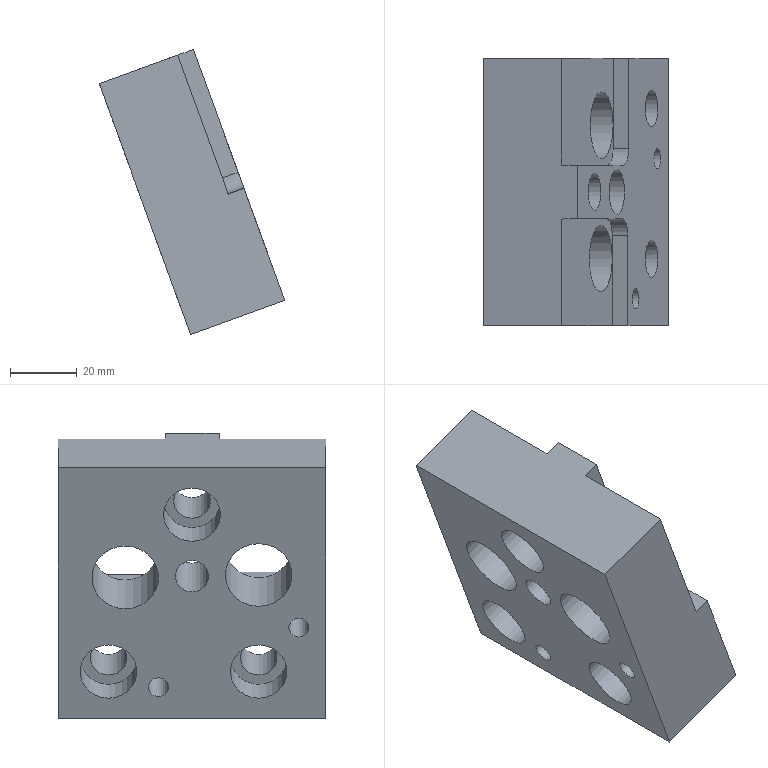Part | NX | features solid 2 | 1 solid | 30 faces | box 55.556 x 80.011 x 85.442 mm | volume 144406 mm3 | plane 16 | cylinder 14 | commonest cylinder face diameters 10 x3 11 x3 17 x3 6 x2 20 x2 13.5 x1
STEP:
#1=CARTESIAN_POINT('',(706.024,-306.997,52.44));
#2=VERTEX_POINT('',#1);
#3=CARTESIAN_POINT('',(703.117,-306.997,60.427));
#4=DIRECTION('',(0.9397,-0.000001517,0.342));
#5=DIRECTION('',(0.342,0.,-0.9397));
#6=AXIS2_PLACEMENT_3D('',#3,#4,#5);
#7=CIRCLE('',#6,8.5);
#8=EDGE_CURVE('',#2,#2,#7,.T.);
#9=ORIENTED_EDGE('',*,*,#8,.T.);
#10=EDGE_LOOP('',(#9));
#11=FACE_BOUND('',#10,.T.);
#12=CARTESIAN_POINT('',(717.31,-281.99,21.433));
#13=VERTEX_POINT('',#12);
#14=CARTESIAN_POINT('',(720.217,-281.99,13.446));
#15=DIRECTION('',(-0.9397,0.000001517,-0.342));
#16=DIRECTION('',(-0.342,0.00000071,0.9397));
#17=AXIS2_PLACEMENT_3D('',#14,#15,#16);
#18=CIRCLE('',#17,8.5);
#19=EDGE_CURVE('',#13,#13,#18,.T.);
#20=ORIENTED_EDGE('',*,*,#19,.F.);
#21=EDGE_LOOP('',(#20));
#22=FACE_BOUND('',#21,.T.);
#23=CARTESIAN_POINT('',(717.312,-326.99,21.427));
#24=VERTEX_POINT('',#23);
#25=CARTESIAN_POINT('',(720.219,-326.99,13.44));
#26=DIRECTION('',(-0.9397,0.000001517,-0.342));
#27=DIRECTION('',(-0.342,0.00000071,0.9397));
#28=AXIS2_PLACEMENT_3D('',#25,#26,#27);
#29=CIRCLE('',#28,8.5);
#30=EDGE_CURVE('',#24,#24,#29,.T.);
#31=ORIENTED_EDGE('',*,*,#30,.F.);
#32=EDGE_LOOP('',(#31));
#33=FACE_BOUND('',#32,.T.);
#34=CARTESIAN_POINT('',(711.536,-306.988,37.297));
#35=VERTEX_POINT('',#34);
#36=CARTESIAN_POINT('',(709.825,-306.988,41.995));
#37=DIRECTION('',(0.9397,-0.000001517,0.342));
#38=DIRECTION('',(0.342,-0.00000071,-0.9397));
#39=AXIS2_PLACEMENT_3D('',#36,#37,#38);
#40=CIRCLE('',#39,5.);
#41=EDGE_CURVE('',#35,#35,#40,.F.);
#42=ORIENTED_EDGE('',*,*,#41,.F.);
#43=EDGE_LOOP('',(#42));
#44=FACE_BOUND('',#43,.T.);
#45=CARTESIAN_POINT('',(725.35,-346.988,-0.6581));
#46=VERTEX_POINT('',#45);
#47=CARTESIAN_POINT('',(697.988,-346.999,74.517));
#48=VERTEX_POINT('',#47);
#49=CARTESIAN_POINT('',(727.06,-346.987,-5.357));
#50=DIRECTION('',(-0.342,-0.0001374,0.9397));
#51=VECTOR('',#50,1000.);
#52=LINE('',#49,#51);
#53=EDGE_CURVE('',#46,#48,#52,.T.);
#54=ORIENTED_EDGE('',*,*,#53,.T.);
#55=CARTESIAN_POINT('',(697.985,-266.999,74.528));
#56=VERTEX_POINT('',#55);
#57=CARTESIAN_POINT('',(697.983,-236.999,74.532));
#58=DIRECTION('',(-0.00004556,1.,0.0001296));
#59=VECTOR('',#58,1000.);
#60=LINE('',#57,#59);
#61=EDGE_CURVE('',#48,#56,#60,.T.);
#62=ORIENTED_EDGE('',*,*,#61,.T.);
#63=CARTESIAN_POINT('',(725.346,-266.988,-0.6477));
#64=VERTEX_POINT('',#63);
#65=CARTESIAN_POINT('',(727.056,-266.987,-5.346));
#66=DIRECTION('',(0.342,0.0001374,-0.9397));
#67=VECTOR('',#66,1000.);
#68=LINE('',#65,#67);
#69=EDGE_CURVE('',#56,#64,#68,.T.);
#70=ORIENTED_EDGE('',*,*,#69,.T.);
#71=CARTESIAN_POINT('',(725.345,-236.988,-0.6438));
#72=DIRECTION('',(0.00004556,-1.,-0.0001296));
#73=VECTOR('',#72,1000.);
#74=LINE('',#71,#73);
#75=EDGE_CURVE('',#64,#46,#74,.T.);
#76=ORIENTED_EDGE('',*,*,#75,.T.);
#77=EDGE_LOOP('',(#54,#62,#70,#76));
#78=FACE_BOUND('',#77,.T.);
#79=CARTESIAN_POINT('',(713.377,-286.994,32.239));
#80=VERTEX_POINT('',#79);
#81=CARTESIAN_POINT('',(709.956,-286.994,41.636));
#82=DIRECTION('',(0.9397,-0.000001517,0.342));
#83=DIRECTION('',(0.342,-0.00000071,-0.9397));
#84=AXIS2_PLACEMENT_3D('',#81,#82,#83);
#85=CIRCLE('',#84,10.);
#86=EDGE_CURVE('',#80,#80,#85,.F.);
#87=ORIENTED_EDGE('',*,*,#86,.F.);
#88=EDGE_LOOP('',(#87));
#89=FACE_BOUND('',#88,.T.);
#90=CARTESIAN_POINT('',(713.111,-326.986,32.967));
#91=VERTEX_POINT('',#90);
#92=CARTESIAN_POINT('',(709.691,-326.986,42.364));
#93=DIRECTION('',(0.9397,-0.000001517,0.342));
#94=DIRECTION('',(0.342,-0.00000071,-0.9397));
#95=AXIS2_PLACEMENT_3D('',#92,#93,#94);
#96=CIRCLE('',#95,10.);
#97=EDGE_CURVE('',#91,#91,#96,.F.);
#98=ORIENTED_EDGE('',*,*,#97,.F.);
#99=EDGE_LOOP('',(#98));
#100=FACE_BOUND('',#99,.T.);
#101=CARTESIAN_POINT('',(722.954,-296.989,5.926));
#102=VERTEX_POINT('',#101);
#103=CARTESIAN_POINT('',(721.927,-296.989,8.745));
#104=DIRECTION('',(0.9397,-0.000001517,0.342));
#105=DIRECTION('',(0.342,0.,-0.9397));
#106=AXIS2_PLACEMENT_3D('',#103,#104,#105);
#107=CIRCLE('',#106,3.);
#108=EDGE_CURVE('',#102,#102,#107,.F.);
#109=ORIENTED_EDGE('',*,*,#108,.F.);
#110=EDGE_LOOP('',(#109));
#111=FACE_BOUND('',#110,.T.);
#112=CARTESIAN_POINT('',(716.457,-338.992,23.775));
#113=VERTEX_POINT('',#112);
#114=CARTESIAN_POINT('',(715.431,-338.992,26.594));
#115=DIRECTION('',(0.9397,-0.000001517,0.342));
#116=DIRECTION('',(0.342,0.,-0.9397));
#117=AXIS2_PLACEMENT_3D('',#114,#115,#116);
#118=CIRCLE('',#117,3.);
#119=EDGE_CURVE('',#113,#113,#118,.F.);
#120=ORIENTED_EDGE('',*,*,#119,.F.);
#121=EDGE_LOOP('',(#120));
#122=FACE_BOUND('',#121,.T.);
#123=CARTESIAN_POINT('',(727.055,-236.987,-5.342));
#124=DIRECTION('',(-0.9397,0.000001517,-0.342));
#125=DIRECTION('',(0.342,0.0001374,-0.9397));
#126=AXIS2_PLACEMENT_3D('',#123,#124,#125);
#127=PLANE('',#126);
#128=ADVANCED_FACE('',(#11,#22,#33,#44,#78,#89,#100,#111,#122),#127,.T.);
#129=CARTESIAN_POINT('',(736.63,-346.993,41.445));
#130=VERTEX_POINT('',#129);
#131=CARTESIAN_POINT('',(721.481,-346.999,83.068));
#132=VERTEX_POINT('',#131);
#133=CARTESIAN_POINT('',(750.552,-346.987,3.194));
#134=DIRECTION('',(-0.342,-0.0001374,0.9397));
#135=VECTOR('',#134,1000.);
#136=LINE('',#133,#135);
#137=EDGE_CURVE('',#130,#132,#136,.T.);
#138=ORIENTED_EDGE('',*,*,#137,.T.);
#139=CARTESIAN_POINT('',(730.878,-346.999,86.488));
#140=DIRECTION('',(-0.9397,0.000001517,-0.342));
#141=VECTOR('',#140,1000.);
#142=LINE('',#139,#141);
#143=EDGE_CURVE('',#132,#48,#142,.T.);
#144=ORIENTED_EDGE('',*,*,#143,.T.);
#145=ORIENTED_EDGE('',*,*,#53,.F.);
#146=CARTESIAN_POINT('',(753.541,-346.988,9.603));
#147=VERTEX_POINT('',#146);
#148=CARTESIAN_POINT('',(758.239,-346.988,11.313));
#149=DIRECTION('',(-0.9397,0.000001517,-0.342));
#150=VECTOR('',#149,1000.);
#151=LINE('',#148,#150);
#152=EDGE_CURVE('',#147,#46,#151,.T.);
#153=ORIENTED_EDGE('',*,*,#152,.F.);
#154=CARTESIAN_POINT('',(741.328,-346.993,43.155));
#155=VERTEX_POINT('',#154);
#156=CARTESIAN_POINT('',(755.251,-346.987,4.904));
#157=DIRECTION('',(0.342,0.0001374,-0.9397));
#158=VECTOR('',#157,1000.);
#159=LINE('',#156,#158);
#160=EDGE_CURVE('',#155,#147,#159,.T.);
#161=ORIENTED_EDGE('',*,*,#160,.F.);
#162=CARTESIAN_POINT('',(736.63,-346.993,41.445));
#163=DIRECTION('',(0.9397,-0.000001517,0.342));
#164=VECTOR('',#163,1000.);
#165=LINE('',#162,#164);
#166=EDGE_CURVE('',#155,#130,#165,.F.);
#167=ORIENTED_EDGE('',*,*,#166,.T.);
#168=EDGE_LOOP('',(#138,#144,#145,#153,#161,#167));
#169=FACE_BOUND('',#168,.T.);
#170=CARTESIAN_POINT('',(759.949,-346.987,6.614));
#171=DIRECTION('',(0.00004556,-1.,-0.0001296));
#172=DIRECTION('',(0.9397,-0.000001517,0.342));
#173=AXIS2_PLACEMENT_3D('',#170,#171,#172);
#174=PLANE('',#173);
#175=ADVANCED_FACE('',(#169),#174,.T.);
#176=CARTESIAN_POINT('',(721.479,-315.154,83.072));
#177=VERTEX_POINT('',#176);
#178=CARTESIAN_POINT('',(721.476,-236.999,83.082));
#179=DIRECTION('',(-0.00004556,1.,0.0001296));
#180=VECTOR('',#179,1000.);
#181=LINE('',#178,#180);
#182=EDGE_CURVE('',#132,#177,#181,.T.);
#183=ORIENTED_EDGE('',*,*,#182,.T.);
#184=CARTESIAN_POINT('',(726.178,-315.154,84.782));
#185=VERTEX_POINT('',#184);
#186=CARTESIAN_POINT('',(730.876,-315.154,86.492));
#187=DIRECTION('',(-0.9397,0.000001517,-0.342));
#188=VECTOR('',#187,1000.);
#189=LINE('',#186,#188);
#190=EDGE_CURVE('',#177,#185,#189,.F.);
#191=ORIENTED_EDGE('',*,*,#190,.T.);
#192=CARTESIAN_POINT('',(726.177,-298.999,84.784));
#193=VERTEX_POINT('',#192);
#194=CARTESIAN_POINT('',(726.174,-236.999,84.792));
#195=DIRECTION('',(0.00004556,-1.,-0.0001296));
#196=VECTOR('',#195,1000.);
#197=LINE('',#194,#196);
#198=EDGE_CURVE('',#193,#185,#197,.T.);
#199=ORIENTED_EDGE('',*,*,#198,.F.);
#200=CARTESIAN_POINT('',(721.479,-298.999,83.074));
#201=VERTEX_POINT('',#200);
#202=CARTESIAN_POINT('',(730.875,-298.999,86.494));
#203=DIRECTION('',(-0.9397,0.000001517,-0.342));
#204=VECTOR('',#203,1000.);
#205=LINE('',#202,#204);
#206=EDGE_CURVE('',#193,#201,#205,.T.);
#207=ORIENTED_EDGE('',*,*,#206,.T.);
#208=CARTESIAN_POINT('',(721.477,-266.999,83.078));
#209=VERTEX_POINT('',#208);
#210=CARTESIAN_POINT('',(721.476,-236.999,83.082));
#211=DIRECTION('',(-0.00004556,1.,0.0001296));
#212=VECTOR('',#211,1000.);
#213=LINE('',#210,#212);
#214=EDGE_CURVE('',#201,#209,#213,.T.);
#215=ORIENTED_EDGE('',*,*,#214,.T.);
#216=CARTESIAN_POINT('',(730.874,-266.999,86.498));
#217=DIRECTION('',(-0.9397,0.000001517,-0.342));
#218=VECTOR('',#217,1000.);
#219=LINE('',#216,#218);
#220=EDGE_CURVE('',#209,#56,#219,.T.);
#221=ORIENTED_EDGE('',*,*,#220,.T.);
#222=ORIENTED_EDGE('',*,*,#61,.F.);
#223=ORIENTED_EDGE('',*,*,#143,.F.);
#224=EDGE_LOOP('',(#183,#191,#199,#207,#215,#221,#222,#223));
#225=FACE_BOUND('',#224,.T.);
#226=CARTESIAN_POINT('',(730.873,-236.999,86.502));
#227=DIRECTION('',(-0.342,-0.0001374,0.9397));
#228=DIRECTION('',(-0.9397,0.000001517,-0.342));
#229=AXIS2_PLACEMENT_3D('',#226,#227,#228);
#230=PLANE('',#229);
#231=ADVANCED_FACE('',(#225),#230,.T.);
#232=CARTESIAN_POINT('',(736.868,-266.993,40.792));
#233=VERTEX_POINT('',#232);
#234=CARTESIAN_POINT('',(750.549,-266.987,3.204));
#235=DIRECTION('',(0.342,0.0001374,-0.9397));
#236=VECTOR('',#235,1000.);
#237=LINE('',#234,#236);
#238=EDGE_CURVE('',#209,#233,#237,.T.);
#239=ORIENTED_EDGE('',*,*,#238,.T.);
#240=CARTESIAN_POINT('',(741.566,-266.993,42.502));
#241=VERTEX_POINT('',#240);
#242=CARTESIAN_POINT('',(746.265,-266.993,44.212));
#243=DIRECTION('',(0.9397,-0.000001517,0.342));
#244=VECTOR('',#243,1000.);
#245=LINE('',#242,#244);
#246=EDGE_CURVE('',#233,#241,#245,.T.);
#247=ORIENTED_EDGE('',*,*,#246,.T.);
#248=CARTESIAN_POINT('',(753.537,-266.988,9.613));
#249=VERTEX_POINT('',#248);
#250=CARTESIAN_POINT('',(755.247,-266.987,4.914));
#251=DIRECTION('',(-0.342,-0.0001374,0.9397));
#252=VECTOR('',#251,1000.);
#253=LINE('',#250,#252);
#254=EDGE_CURVE('',#249,#241,#253,.T.);
#255=ORIENTED_EDGE('',*,*,#254,.F.);
#256=CARTESIAN_POINT('',(758.236,-266.988,11.323));
#257=DIRECTION('',(-0.9397,0.000001517,-0.342));
#258=VECTOR('',#257,1000.);
#259=LINE('',#256,#258);
#260=EDGE_CURVE('',#249,#64,#259,.T.);
#261=ORIENTED_EDGE('',*,*,#260,.T.);
#262=ORIENTED_EDGE('',*,*,#69,.F.);
#263=ORIENTED_EDGE('',*,*,#220,.F.);
#264=EDGE_LOOP('',(#239,#247,#255,#261,#262,#263));
#265=FACE_BOUND('',#264,.T.);
#266=CARTESIAN_POINT('',(759.946,-266.987,6.625));
#267=DIRECTION('',(-0.00004556,1.,0.0001296));
#268=DIRECTION('',(-0.9397,0.000001517,-0.342));
#269=AXIS2_PLACEMENT_3D('',#266,#267,#268);
#270=PLANE('',#269);
#271=ADVANCED_FACE('',(#265),#270,.T.);
#272=CARTESIAN_POINT('',(729.427,-306.997,75.856));
#273=VERTEX_POINT('',#272);
#274=CARTESIAN_POINT('',(731.308,-306.997,70.688));
#275=DIRECTION('',(-0.9397,0.000001517,-0.342));
#276=DIRECTION('',(-0.342,0.,0.9397));
#277=AXIS2_PLACEMENT_3D('',#274,#275,#276);
#278=CIRCLE('',#277,5.5);
#279=EDGE_CURVE('',#273,#273,#278,.T.);
#280=ORIENTED_EDGE('',*,*,#279,.T.);
#281=EDGE_LOOP('',(#280));
#282=FACE_BOUND('',#281,.T.);
#283=CARTESIAN_POINT('',(742.596,-338.992,39.674));
#284=VERTEX_POINT('',#283);
#285=CARTESIAN_POINT('',(743.622,-338.992,36.855));
#286=DIRECTION('',(-0.9397,0.000001517,-0.342));
#287=DIRECTION('',(-0.342,0.00000071,0.9397));
#288=AXIS2_PLACEMENT_3D('',#285,#286,#287);
#289=CIRCLE('',#288,3.);
#290=EDGE_CURVE('',#284,#284,#289,.T.);
#291=ORIENTED_EDGE('',*,*,#290,.T.);
#292=EDGE_LOOP('',(#291));
#293=FACE_BOUND('',#292,.T.);
#294=CARTESIAN_POINT('',(749.092,-296.989,21.825));
#295=VERTEX_POINT('',#294);
#296=CARTESIAN_POINT('',(750.118,-296.989,19.006));
#297=DIRECTION('',(-0.9397,0.000001517,-0.342));
#298=DIRECTION('',(-0.342,0.00000071,0.9397));
#299=AXIS2_PLACEMENT_3D('',#296,#297,#298);
#300=CIRCLE('',#299,3.);
#301=EDGE_CURVE('',#295,#295,#300,.T.);
#302=ORIENTED_EDGE('',*,*,#301,.T.);
#303=EDGE_LOOP('',(#302));
#304=FACE_BOUND('',#303,.T.);
#305=CARTESIAN_POINT('',(746.526,-281.99,28.875));
#306=VERTEX_POINT('',#305);
#307=CARTESIAN_POINT('',(748.407,-281.99,23.706));
#308=DIRECTION('',(-0.9397,0.000001517,-0.342));
#309=DIRECTION('',(-0.342,0.00000071,0.9397));
#310=AXIS2_PLACEMENT_3D('',#307,#308,#309);
#311=CIRCLE('',#310,5.5);
#312=EDGE_CURVE('',#306,#306,#311,.T.);
#313=ORIENTED_EDGE('',*,*,#312,.T.);
#314=EDGE_LOOP('',(#313));
#315=FACE_BOUND('',#314,.T.);
#316=CARTESIAN_POINT('',(746.528,-326.99,28.869));
#317=VERTEX_POINT('',#316);
#318=CARTESIAN_POINT('',(748.41,-326.99,23.701));
#319=DIRECTION('',(-0.9397,0.000001517,-0.342));
#320=DIRECTION('',(-0.342,0.00000071,0.9397));
#321=AXIS2_PLACEMENT_3D('',#318,#319,#320);
#322=CIRCLE('',#321,5.5);
#323=EDGE_CURVE('',#317,#317,#322,.T.);
#324=ORIENTED_EDGE('',*,*,#323,.T.);
#325=EDGE_LOOP('',(#324));
#326=FACE_BOUND('',#325,.T.);
#327=ORIENTED_EDGE('',*,*,#160,.T.);
#328=CARTESIAN_POINT('',(753.536,-236.988,9.617));
#329=DIRECTION('',(-0.00004556,1.,0.0001296));
#330=VECTOR('',#329,1000.);
#331=LINE('',#328,#330);
#332=EDGE_CURVE('',#147,#249,#331,.T.);
#333=ORIENTED_EDGE('',*,*,#332,.T.);
#334=ORIENTED_EDGE('',*,*,#254,.T.);
#335=CARTESIAN_POINT('',(741.568,-293.993,42.499));
#336=VERTEX_POINT('',#335);
#337=CARTESIAN_POINT('',(741.565,-236.993,42.506));
#338=DIRECTION('',(0.00004556,-1.,-0.0001296));
#339=VECTOR('',#338,1000.);
#340=LINE('',#337,#339);
#341=EDGE_CURVE('',#241,#336,#340,.T.);
#342=ORIENTED_EDGE('',*,*,#341,.T.);
#343=CARTESIAN_POINT('',(739.858,-298.993,47.196));
#344=VERTEX_POINT('',#343);
#345=CARTESIAN_POINT('',(739.858,-293.993,47.197));
#346=DIRECTION('',(-0.9397,0.000001517,-0.342));
#347=DIRECTION('',(-0.342,0.00000071,0.9397));
#348=AXIS2_PLACEMENT_3D('',#345,#346,#347);
#349=CIRCLE('',#348,5.);
#350=EDGE_CURVE('',#344,#336,#349,.F.);
#351=ORIENTED_EDGE('',*,*,#350,.F.);
#352=CARTESIAN_POINT('',(755.249,-298.987,4.91));
#353=DIRECTION('',(-0.342,-0.0001374,0.9397));
#354=VECTOR('',#353,1000.);
#355=LINE('',#352,#354);
#356=EDGE_CURVE('',#344,#193,#355,.T.);
#357=ORIENTED_EDGE('',*,*,#356,.T.);
#358=ORIENTED_EDGE('',*,*,#198,.T.);
#359=CARTESIAN_POINT('',(739.576,-315.004,47.969));
#360=VERTEX_POINT('',#359);
#361=CARTESIAN_POINT('',(755.348,-314.827,4.638));
#362=DIRECTION('',(-0.342,-0.003837,0.9397));
#363=VECTOR('',#362,1000.);
#364=LINE('',#361,#363);
#365=EDGE_CURVE('',#185,#360,#364,.F.);
#366=ORIENTED_EDGE('',*,*,#365,.T.);
#367=CARTESIAN_POINT('',(741.293,-319.985,43.253));
#368=VERTEX_POINT('',#367);
#369=CARTESIAN_POINT('',(739.583,-320.004,47.951));
#370=DIRECTION('',(-0.9397,0.000001517,-0.342));
#371=DIRECTION('',(-0.342,0.00000071,0.9397));
#372=AXIS2_PLACEMENT_3D('',#369,#370,#371);
#373=CIRCLE('',#372,5.);
#374=EDGE_CURVE('',#368,#360,#373,.F.);
#375=ORIENTED_EDGE('',*,*,#374,.F.);
#376=CARTESIAN_POINT('',(741.275,-306.392,43.302));
#377=DIRECTION('',(-0.001311,1.,0.003606));
#378=VECTOR('',#377,1000.);
#379=LINE('',#376,#378);
#380=EDGE_CURVE('',#368,#155,#379,.F.);
#381=ORIENTED_EDGE('',*,*,#380,.T.);
#382=EDGE_LOOP('',(#327,#333,#334,#342,#351,#357,#358,#366,#375,#381));
#383=FACE_BOUND('',#382,.T.);
#384=CARTESIAN_POINT('',(735.708,-306.989,58.599));
#385=VERTEX_POINT('',#384);
#386=CARTESIAN_POINT('',(738.016,-306.989,52.256));
#387=DIRECTION('',(-0.9397,0.000001517,-0.342));
#388=DIRECTION('',(-0.342,0.00000071,0.9397));
#389=AXIS2_PLACEMENT_3D('',#386,#387,#388);
#390=CIRCLE('',#389,6.75);
#391=EDGE_CURVE('',#385,#385,#390,.T.);
#392=ORIENTED_EDGE('',*,*,#391,.T.);
#393=EDGE_LOOP('',(#392));
#394=FACE_BOUND('',#393,.T.);
#395=CARTESIAN_POINT('',(755.246,-236.987,4.918));
#396=DIRECTION('',(0.9397,-0.000001517,0.342));
#397=DIRECTION('',(-0.342,-0.0001374,0.9397));
#398=AXIS2_PLACEMENT_3D('',#395,#396,#397);
#399=PLANE('',#398);
#400=ADVANCED_FACE('',(#282,#293,#304,#315,#326,#383,#394),#399,.T.);
#401=ORIENTED_EDGE('',*,*,#332,.F.);
#402=ORIENTED_EDGE('',*,*,#152,.T.);
#403=ORIENTED_EDGE('',*,*,#75,.F.);
#404=ORIENTED_EDGE('',*,*,#260,.F.);
#405=EDGE_LOOP('',(#401,#402,#403,#404));
#406=FACE_BOUND('',#405,.T.);
#407=CARTESIAN_POINT('',(758.234,-236.988,11.327));
#408=DIRECTION('',(0.342,0.0001374,-0.9397));
#409=DIRECTION('',(0.9397,-0.000001517,0.342));
#410=AXIS2_PLACEMENT_3D('',#407,#408,#409);
#411=PLANE('',#410);
#412=ADVANCED_FACE('',(#406),#411,.T.);
#413=CARTESIAN_POINT('',(736.869,-286.993,40.789));
#414=VERTEX_POINT('',#413);
#415=CARTESIAN_POINT('',(736.869,-293.993,40.789));
#416=VERTEX_POINT('',#415);
#417=CARTESIAN_POINT('',(736.869,-281.993,40.79));
#418=DIRECTION('',(0.00004556,-1.,-0.0001296));
#419=VECTOR('',#418,1000.);
#420=LINE('',#417,#419);
#421=EDGE_CURVE('',#414,#416,#420,.T.);
#422=ORIENTED_EDGE('',*,*,#421,.F.);
#423=CARTESIAN_POINT('',(733.449,-286.994,50.186));
#424=DIRECTION('',(-0.9397,0.000001517,-0.342));
#425=DIRECTION('',(-0.342,-0.0001374,0.9397));
#426=AXIS2_PLACEMENT_3D('',#423,#424,#425);
#427=CIRCLE('',#426,10.);
#428=EDGE_CURVE('',#414,#414,#427,.T.);
#429=ORIENTED_EDGE('',*,*,#428,.T.);
#430=CARTESIAN_POINT('',(736.869,-281.993,40.79));
#431=DIRECTION('',(0.00004556,-1.,-0.0001296));
#432=VECTOR('',#431,1000.);
#433=LINE('',#430,#432);
#434=EDGE_CURVE('',#233,#414,#433,.T.);
#435=ORIENTED_EDGE('',*,*,#434,.F.);
#436=ORIENTED_EDGE('',*,*,#238,.F.);
#437=ORIENTED_EDGE('',*,*,#214,.F.);
#438=CARTESIAN_POINT('',(735.159,-298.993,45.486));
#439=VERTEX_POINT('',#438);
#440=CARTESIAN_POINT('',(735.159,-298.993,45.486));
#441=DIRECTION('',(-0.342,-0.0001374,0.9397));
#442=VECTOR('',#441,1000.);
#443=LINE('',#440,#442);
#444=EDGE_CURVE('',#439,#201,#443,.T.);
#445=ORIENTED_EDGE('',*,*,#444,.F.);
#446=CARTESIAN_POINT('',(735.159,-293.993,45.487));
#447=DIRECTION('',(0.9397,-0.000001517,0.342));
#448=DIRECTION('',(0.342,-0.00000071,-0.9397));
#449=AXIS2_PLACEMENT_3D('',#446,#447,#448);
#450=CIRCLE('',#449,5.);
#451=EDGE_CURVE('',#416,#439,#450,.F.);
#452=ORIENTED_EDGE('',*,*,#451,.F.);
#453=EDGE_LOOP('',(#422,#429,#435,#436,#437,#445,#452));
#454=FACE_BOUND('',#453,.T.);
#455=CARTESIAN_POINT('',(735.159,-281.993,45.489));
#456=DIRECTION('',(-0.9397,0.000001517,-0.342));
#457=DIRECTION('',(0.342,0.0001374,-0.9397));
#458=AXIS2_PLACEMENT_3D('',#455,#456,#457);
#459=PLANE('',#458);
#460=ADVANCED_FACE('',(#454),#459,.F.);
#461=ORIENTED_EDGE('',*,*,#444,.T.);
#462=ORIENTED_EDGE('',*,*,#206,.F.);
#463=ORIENTED_EDGE('',*,*,#356,.F.);
#464=CARTESIAN_POINT('',(739.858,-298.993,47.196));
#465=DIRECTION('',(-0.9397,0.000001517,-0.342));
#466=VECTOR('',#465,1000.);
#467=LINE('',#464,#466);
#468=EDGE_CURVE('',#439,#344,#467,.F.);
#469=ORIENTED_EDGE('',*,*,#468,.F.);
#470=EDGE_LOOP('',(#461,#462,#463,#469));
#471=FACE_BOUND('',#470,.T.);
#472=CARTESIAN_POINT('',(739.858,-298.993,47.196));
#473=DIRECTION('',(0.00004556,-1.,-0.0001296));
#474=DIRECTION('',(0.9397,-0.000001517,0.342));
#475=AXIS2_PLACEMENT_3D('',#472,#473,#474);
#476=PLANE('',#475);
#477=ADVANCED_FACE('',(#471),#476,.F.);
#478=ORIENTED_EDGE('',*,*,#341,.F.);
#479=ORIENTED_EDGE('',*,*,#246,.F.);
#480=ORIENTED_EDGE('',*,*,#434,.T.);
#481=ORIENTED_EDGE('',*,*,#421,.T.);
#482=CARTESIAN_POINT('',(736.869,-293.993,40.789));
#483=DIRECTION('',(-0.9397,0.000001517,-0.342));
#484=VECTOR('',#483,1000.);
#485=LINE('',#482,#484);
#486=EDGE_CURVE('',#336,#416,#485,.T.);
#487=ORIENTED_EDGE('',*,*,#486,.F.);
#488=EDGE_LOOP('',(#478,#479,#480,#481,#487));
#489=FACE_BOUND('',#488,.T.);
#490=CARTESIAN_POINT('',(741.567,-281.993,42.5));
#491=DIRECTION('',(0.342,0.0001374,-0.9397));
#492=DIRECTION('',(0.9397,-0.000001517,0.342));
#493=AXIS2_PLACEMENT_3D('',#490,#491,#492);
#494=PLANE('',#493);
#495=ADVANCED_FACE('',(#489),#494,.F.);
#496=CARTESIAN_POINT('',(734.878,-315.004,46.259));
#497=VERTEX_POINT('',#496);
#498=CARTESIAN_POINT('',(736.588,-314.985,41.561));
#499=DIRECTION('',(-0.342,-0.003837,0.9397));
#500=VECTOR('',#499,1000.);
#501=LINE('',#498,#500);
#502=EDGE_CURVE('',#177,#497,#501,.F.);
#503=ORIENTED_EDGE('',*,*,#502,.F.);
#504=ORIENTED_EDGE('',*,*,#182,.F.);
#505=ORIENTED_EDGE('',*,*,#137,.F.);
#506=CARTESIAN_POINT('',(736.604,-326.948,41.518));
#507=VERTEX_POINT('',#506);
#508=CARTESIAN_POINT('',(736.597,-321.966,41.536));
#509=DIRECTION('',(-0.001311,1.,0.003606));
#510=VECTOR('',#509,1000.);
#511=LINE('',#508,#510);
#512=EDGE_CURVE('',#507,#130,#511,.F.);
#513=ORIENTED_EDGE('',*,*,#512,.F.);
#514=CARTESIAN_POINT('',(733.184,-326.986,50.914));
#515=DIRECTION('',(-0.9397,0.000001517,-0.342));
#516=DIRECTION('',(-0.342,-0.003837,0.9397));
#517=AXIS2_PLACEMENT_3D('',#514,#515,#516);
#518=CIRCLE('',#517,10.);
#519=EDGE_CURVE('',#507,#507,#518,.T.);
#520=ORIENTED_EDGE('',*,*,#519,.T.);
#521=CARTESIAN_POINT('',(736.595,-319.985,41.543));
#522=VERTEX_POINT('',#521);
#523=CARTESIAN_POINT('',(736.597,-321.966,41.536));
#524=DIRECTION('',(-0.001311,1.,0.003606));
#525=VECTOR('',#524,1000.);
#526=LINE('',#523,#525);
#527=EDGE_CURVE('',#522,#507,#526,.F.);
#528=ORIENTED_EDGE('',*,*,#527,.F.);
#529=CARTESIAN_POINT('',(734.885,-320.004,46.241));
#530=DIRECTION('',(0.9397,-0.000001517,0.342));
#531=DIRECTION('',(0.342,-0.00000071,-0.9397));
#532=AXIS2_PLACEMENT_3D('',#529,#530,#531);
#533=CIRCLE('',#532,5.);
#534=EDGE_CURVE('',#497,#522,#533,.F.);
#535=ORIENTED_EDGE('',*,*,#534,.F.);
#536=EDGE_LOOP('',(#503,#504,#505,#513,#520,#528,#535));
#537=FACE_BOUND('',#536,.T.);
#538=CARTESIAN_POINT('',(734.893,-321.985,46.217));
#539=DIRECTION('',(-0.9397,0.000001517,-0.342));
#540=DIRECTION('',(0.342,0.0001374,-0.9397));
#541=AXIS2_PLACEMENT_3D('',#538,#539,#540);
#542=PLANE('',#541);
#543=ADVANCED_FACE('',(#537),#542,.F.);
#544=ORIENTED_EDGE('',*,*,#365,.F.);
#545=ORIENTED_EDGE('',*,*,#190,.F.);
#546=ORIENTED_EDGE('',*,*,#502,.T.);
#547=CARTESIAN_POINT('',(734.878,-315.004,46.259));
#548=DIRECTION('',(0.9397,-0.000001517,0.342));
#549=VECTOR('',#548,1000.);
#550=LINE('',#547,#549);
#551=EDGE_CURVE('',#360,#497,#550,.F.);
#552=ORIENTED_EDGE('',*,*,#551,.F.);
#553=EDGE_LOOP('',(#544,#545,#546,#552));
#554=FACE_BOUND('',#553,.T.);
#555=CARTESIAN_POINT('',(736.588,-314.985,41.561));
#556=DIRECTION('',(0.001311,-1.,-0.003606));
#557=DIRECTION('',(-0.000000496,0.003606,-1.));
#558=AXIS2_PLACEMENT_3D('',#555,#556,#557);
#559=PLANE('',#558);
#560=ADVANCED_FACE('',(#554),#559,.T.);
#561=ORIENTED_EDGE('',*,*,#527,.T.);
#562=ORIENTED_EDGE('',*,*,#512,.T.);
#563=ORIENTED_EDGE('',*,*,#166,.F.);
#564=ORIENTED_EDGE('',*,*,#380,.F.);
#565=CARTESIAN_POINT('',(736.595,-319.985,41.543));
#566=DIRECTION('',(0.9397,-0.000001517,0.342));
#567=VECTOR('',#566,1000.);
#568=LINE('',#565,#567);
#569=EDGE_CURVE('',#522,#368,#568,.T.);
#570=ORIENTED_EDGE('',*,*,#569,.F.);
#571=EDGE_LOOP('',(#561,#562,#563,#564,#570));
#572=FACE_BOUND('',#571,.T.);
#573=CARTESIAN_POINT('',(736.577,-306.392,41.592));
#574=DIRECTION('',(0.342,0.003837,-0.9397));
#575=DIRECTION('',(0.001311,-1.,-0.003606));
#576=AXIS2_PLACEMENT_3D('',#573,#574,#575);
#577=PLANE('',#576);
#578=ADVANCED_FACE('',(#572),#577,.F.);
#579=ORIENTED_EDGE('',*,*,#391,.F.);
#580=EDGE_LOOP('',(#579));
#581=FACE_BOUND('',#580,.T.);
#582=CARTESIAN_POINT('',(735.626,-306.989,44.203));
#583=VERTEX_POINT('',#582);
#584=CARTESIAN_POINT('',(733.318,-306.989,50.546));
#585=DIRECTION('',(0.9397,-0.000001517,0.342));
#586=DIRECTION('',(0.342,-0.00000071,-0.9397));
#587=AXIS2_PLACEMENT_3D('',#584,#585,#586);
#588=CIRCLE('',#587,6.75);
#589=EDGE_CURVE('',#583,#583,#588,.T.);
#590=ORIENTED_EDGE('',*,*,#589,.F.);
#591=EDGE_LOOP('',(#590));
#592=FACE_BOUND('',#591,.T.);
#593=CARTESIAN_POINT('',(742.715,-306.989,53.966));
#594=DIRECTION('',(-0.9397,0.000001517,-0.342));
#595=DIRECTION('',(0.342,-0.00000071,-0.9397));
#596=AXIS2_PLACEMENT_3D('',#593,#594,#595);
#597=CYLINDRICAL_SURFACE('',#596,6.75);
#598=ADVANCED_FACE('',(#581,#592),#597,.F.);
#599=ORIENTED_EDGE('',*,*,#589,.T.);
#600=EDGE_LOOP('',(#599));
#601=FACE_BOUND('',#600,.T.);
#602=CARTESIAN_POINT('',(731.608,-306.989,55.244));
#603=VERTEX_POINT('',#602);
#604=CARTESIAN_POINT('',(733.318,-306.989,50.546));
#605=DIRECTION('',(-0.9397,0.000001517,-0.342));
#606=DIRECTION('',(-0.342,0.00000071,0.9397));
#607=AXIS2_PLACEMENT_3D('',#604,#605,#606);
#608=CIRCLE('',#607,5.);
#609=EDGE_CURVE('',#603,#603,#608,.T.);
#610=ORIENTED_EDGE('',*,*,#609,.T.);
#611=EDGE_LOOP('',(#610));
#612=FACE_BOUND('',#611,.T.);
#613=CARTESIAN_POINT('',(733.318,-306.989,50.546));
#614=DIRECTION('',(-0.9397,0.000001517,-0.342));
#615=DIRECTION('',(0.342,-0.00000071,-0.9397));
#616=AXIS2_PLACEMENT_3D('',#613,#614,#615);
#617=PLANE('',#616);
#618=ADVANCED_FACE('',(#601,#612),#617,.F.);
#619=ORIENTED_EDGE('',*,*,#86,.T.);
#620=EDGE_LOOP('',(#619));
#621=FACE_BOUND('',#620,.T.);
#622=ORIENTED_EDGE('',*,*,#428,.F.);
#623=EDGE_LOOP('',(#622));
#624=FACE_BOUND('',#623,.T.);
#625=CARTESIAN_POINT('',(738.147,-286.994,51.896));
#626=DIRECTION('',(-0.9397,0.000001517,-0.342));
#627=DIRECTION('',(0.342,0.0001374,-0.9397));
#628=AXIS2_PLACEMENT_3D('',#625,#626,#627);
#629=CYLINDRICAL_SURFACE('',#628,10.);
#630=ADVANCED_FACE('',(#621,#624),#629,.F.);
#631=ORIENTED_EDGE('',*,*,#41,.T.);
#632=EDGE_LOOP('',(#631));
#633=FACE_BOUND('',#632,.T.);
#634=ORIENTED_EDGE('',*,*,#609,.F.);
#635=EDGE_LOOP('',(#634));
#636=FACE_BOUND('',#635,.T.);
#637=CARTESIAN_POINT('',(738.016,-306.989,52.256));
#638=DIRECTION('',(-0.9397,0.000001517,-0.342));
#639=DIRECTION('',(0.342,-0.00000071,-0.9397));
#640=AXIS2_PLACEMENT_3D('',#637,#638,#639);
#641=CYLINDRICAL_SURFACE('',#640,5.);
#642=ADVANCED_FACE('',(#633,#636),#641,.F.);
#643=ORIENTED_EDGE('',*,*,#97,.T.);
#644=EDGE_LOOP('',(#643));
#645=FACE_BOUND('',#644,.T.);
#646=ORIENTED_EDGE('',*,*,#519,.F.);
#647=EDGE_LOOP('',(#646));
#648=FACE_BOUND('',#647,.T.);
#649=CARTESIAN_POINT('',(737.882,-326.986,52.625));
#650=DIRECTION('',(-0.9397,0.000001517,-0.342));
#651=DIRECTION('',(0.342,0.003837,-0.9397));
#652=AXIS2_PLACEMENT_3D('',#649,#650,#651);
#653=CYLINDRICAL_SURFACE('',#652,10.);
#654=ADVANCED_FACE('',(#645,#648),#653,.F.);
#655=ORIENTED_EDGE('',*,*,#323,.F.);
#656=EDGE_LOOP('',(#655));
#657=FACE_BOUND('',#656,.T.);
#658=CARTESIAN_POINT('',(729.614,-326.99,22.712));
#659=VERTEX_POINT('',#658);
#660=CARTESIAN_POINT('',(731.495,-326.99,17.544));
#661=DIRECTION('',(-0.9397,0.000001517,-0.342));
#662=DIRECTION('',(-0.342,0.00000071,0.9397));
#663=AXIS2_PLACEMENT_3D('',#660,#661,#662);
#664=CIRCLE('',#663,5.5);
#665=EDGE_CURVE('',#659,#659,#664,.T.);
#666=ORIENTED_EDGE('',*,*,#665,.T.);
#667=EDGE_LOOP('',(#666));
#668=FACE_BOUND('',#667,.T.);
#669=CARTESIAN_POINT('',(767.203,-326.99,30.541));
#670=DIRECTION('',(0.9397,-0.000001517,0.342));
#671=DIRECTION('',(-0.342,0.00000071,0.9397));
#672=AXIS2_PLACEMENT_3D('',#669,#670,#671);
#673=CYLINDRICAL_SURFACE('',#672,5.5);
#674=ADVANCED_FACE('',(#657,#668),#673,.F.);
#675=ORIENTED_EDGE('',*,*,#665,.F.);
#676=EDGE_LOOP('',(#675));
#677=FACE_BOUND('',#676,.T.);
#678=CARTESIAN_POINT('',(728.588,-326.99,25.532));
#679=VERTEX_POINT('',#678);
#680=CARTESIAN_POINT('',(731.495,-326.99,17.544));
#681=DIRECTION('',(-0.9397,0.000001517,-0.342));
#682=DIRECTION('',(-0.342,0.00000071,0.9397));
#683=AXIS2_PLACEMENT_3D('',#680,#681,#682);
#684=CIRCLE('',#683,8.5);
#685=EDGE_CURVE('',#679,#679,#684,.T.);
#686=ORIENTED_EDGE('',*,*,#685,.T.);
#687=EDGE_LOOP('',(#686));
#688=FACE_BOUND('',#687,.T.);
#689=CARTESIAN_POINT('',(731.495,-326.99,17.544));
#690=DIRECTION('',(0.9397,-0.000001517,0.342));
#691=DIRECTION('',(-0.342,0.00000071,0.9397));
#692=AXIS2_PLACEMENT_3D('',#689,#690,#691);
#693=PLANE('',#692);
#694=ADVANCED_FACE('',(#677,#688),#693,.F.);
#695=ORIENTED_EDGE('',*,*,#685,.F.);
#696=EDGE_LOOP('',(#695));
#697=FACE_BOUND('',#696,.T.);
#698=ORIENTED_EDGE('',*,*,#30,.T.);
#699=EDGE_LOOP('',(#698));
#700=FACE_BOUND('',#699,.T.);
#701=CARTESIAN_POINT('',(720.219,-326.99,13.44));
#702=DIRECTION('',(0.9397,-0.000001517,0.342));
#703=DIRECTION('',(-0.342,0.00000071,0.9397));
#704=AXIS2_PLACEMENT_3D('',#701,#702,#703);
#705=CYLINDRICAL_SURFACE('',#704,8.5);
#706=ADVANCED_FACE('',(#697,#700),#705,.F.);
#707=ORIENTED_EDGE('',*,*,#312,.F.);
#708=EDGE_LOOP('',(#707));
#709=FACE_BOUND('',#708,.T.);
#710=CARTESIAN_POINT('',(729.612,-281.99,22.718));
#711=VERTEX_POINT('',#710);
#712=CARTESIAN_POINT('',(731.493,-281.99,17.55));
#713=DIRECTION('',(-0.9397,0.000001517,-0.342));
#714=DIRECTION('',(-0.342,0.00000071,0.9397));
#715=AXIS2_PLACEMENT_3D('',#712,#713,#714);
#716=CIRCLE('',#715,5.5);
#717=EDGE_CURVE('',#711,#711,#716,.T.);
#718=ORIENTED_EDGE('',*,*,#717,.T.);
#719=EDGE_LOOP('',(#718));
#720=FACE_BOUND('',#719,.T.);
#721=CARTESIAN_POINT('',(767.201,-281.99,30.547));
#722=DIRECTION('',(0.9397,-0.000001517,0.342));
#723=DIRECTION('',(-0.342,0.00000071,0.9397));
#724=AXIS2_PLACEMENT_3D('',#721,#722,#723);
#725=CYLINDRICAL_SURFACE('',#724,5.5);
#726=ADVANCED_FACE('',(#709,#720),#725,.F.);
#727=ORIENTED_EDGE('',*,*,#717,.F.);
#728=EDGE_LOOP('',(#727));
#729=FACE_BOUND('',#728,.T.);
#730=CARTESIAN_POINT('',(728.586,-281.99,25.537));
#731=VERTEX_POINT('',#730);
#732=CARTESIAN_POINT('',(731.493,-281.99,17.55));
#733=DIRECTION('',(-0.9397,0.000001517,-0.342));
#734=DIRECTION('',(-0.342,0.00000071,0.9397));
#735=AXIS2_PLACEMENT_3D('',#732,#733,#734);
#736=CIRCLE('',#735,8.5);
#737=EDGE_CURVE('',#731,#731,#736,.T.);
#738=ORIENTED_EDGE('',*,*,#737,.T.);
#739=EDGE_LOOP('',(#738));
#740=FACE_BOUND('',#739,.T.);
#741=CARTESIAN_POINT('',(731.493,-281.99,17.55));
#742=DIRECTION('',(0.9397,-0.000001517,0.342));
#743=DIRECTION('',(-0.342,0.00000071,0.9397));
#744=AXIS2_PLACEMENT_3D('',#741,#742,#743);
#745=PLANE('',#744);
#746=ADVANCED_FACE('',(#729,#740),#745,.F.);
#747=ORIENTED_EDGE('',*,*,#737,.F.);
#748=EDGE_LOOP('',(#747));
#749=FACE_BOUND('',#748,.T.);
#750=ORIENTED_EDGE('',*,*,#19,.T.);
#751=EDGE_LOOP('',(#750));
#752=FACE_BOUND('',#751,.T.);
#753=CARTESIAN_POINT('',(720.217,-281.99,13.446));
#754=DIRECTION('',(0.9397,-0.000001517,0.342));
#755=DIRECTION('',(-0.342,0.00000071,0.9397));
#756=AXIS2_PLACEMENT_3D('',#753,#754,#755);
#757=CYLINDRICAL_SURFACE('',#756,8.5);
#758=ADVANCED_FACE('',(#749,#752),#757,.F.);
#759=ORIENTED_EDGE('',*,*,#301,.F.);
#760=EDGE_LOOP('',(#759));
#761=FACE_BOUND('',#760,.T.);
#762=ORIENTED_EDGE('',*,*,#108,.T.);
#763=EDGE_LOOP('',(#762));
#764=FACE_BOUND('',#763,.T.);
#765=CARTESIAN_POINT('',(768.912,-296.989,25.846));
#766=DIRECTION('',(0.9397,-0.000001517,0.342));
#767=DIRECTION('',(-0.342,0.00000071,0.9397));
#768=AXIS2_PLACEMENT_3D('',#765,#766,#767);
#769=CYLINDRICAL_SURFACE('',#768,3.);
#770=ADVANCED_FACE('',(#761,#764),#769,.F.);
#771=ORIENTED_EDGE('',*,*,#290,.F.);
#772=EDGE_LOOP('',(#771));
#773=FACE_BOUND('',#772,.T.);
#774=ORIENTED_EDGE('',*,*,#119,.T.);
#775=EDGE_LOOP('',(#774));
#776=FACE_BOUND('',#775,.T.);
#777=CARTESIAN_POINT('',(762.416,-338.992,43.695));
#778=DIRECTION('',(0.9397,-0.000001517,0.342));
#779=DIRECTION('',(-0.342,0.00000071,0.9397));
#780=AXIS2_PLACEMENT_3D('',#777,#778,#779);
#781=CYLINDRICAL_SURFACE('',#780,3.);
#782=ADVANCED_FACE('',(#773,#776),#781,.F.);
#783=ORIENTED_EDGE('',*,*,#350,.T.);
#784=ORIENTED_EDGE('',*,*,#486,.T.);
#785=ORIENTED_EDGE('',*,*,#451,.T.);
#786=ORIENTED_EDGE('',*,*,#468,.T.);
#787=EDGE_LOOP('',(#783,#784,#785,#786));
#788=FACE_BOUND('',#787,.T.);
#789=CARTESIAN_POINT('',(739.858,-293.993,47.197));
#790=DIRECTION('',(0.9397,-0.000001517,0.342));
#791=DIRECTION('',(-0.342,0.00000071,0.9397));
#792=AXIS2_PLACEMENT_3D('',#789,#790,#791);
#793=CYLINDRICAL_SURFACE('',#792,5.);
#794=ADVANCED_FACE('',(#788),#793,.F.);
#795=ORIENTED_EDGE('',*,*,#374,.T.);
#796=ORIENTED_EDGE('',*,*,#551,.T.);
#797=ORIENTED_EDGE('',*,*,#534,.T.);
#798=ORIENTED_EDGE('',*,*,#569,.T.);
#799=EDGE_LOOP('',(#795,#796,#797,#798));
#800=FACE_BOUND('',#799,.T.);
#801=CARTESIAN_POINT('',(734.885,-320.004,46.241));
#802=DIRECTION('',(-0.9397,0.000001517,-0.342));
#803=DIRECTION('',(0.342,-0.00000071,-0.9397));
#804=AXIS2_PLACEMENT_3D('',#801,#802,#803);
#805=CYLINDRICAL_SURFACE('',#804,5.);
#806=ADVANCED_FACE('',(#800),#805,.F.);
#807=ORIENTED_EDGE('',*,*,#279,.F.);
#808=EDGE_LOOP('',(#807));
#809=FACE_BOUND('',#808,.T.);
#810=CARTESIAN_POINT('',(712.512,-306.997,69.7));
#811=VERTEX_POINT('',#810);
#812=CARTESIAN_POINT('',(714.393,-306.997,64.531));
#813=DIRECTION('',(-0.9397,0.000001517,-0.342));
#814=DIRECTION('',(-0.342,0.,0.9397));
#815=AXIS2_PLACEMENT_3D('',#812,#813,#814);
#816=CIRCLE('',#815,5.5);
#817=EDGE_CURVE('',#811,#811,#816,.F.);
#818=ORIENTED_EDGE('',*,*,#817,.F.);
#819=EDGE_LOOP('',(#818));
#820=FACE_BOUND('',#819,.T.);
#821=CARTESIAN_POINT('',(748.222,-306.997,76.844));
#822=DIRECTION('',(-0.9397,0.000001517,-0.342));
#823=DIRECTION('',(0.342,0.,-0.9397));
#824=AXIS2_PLACEMENT_3D('',#821,#822,#823);
#825=CYLINDRICAL_SURFACE('',#824,5.5);
#826=ADVANCED_FACE('',(#809,#820),#825,.F.);
#827=ORIENTED_EDGE('',*,*,#817,.T.);
#828=EDGE_LOOP('',(#827));
#829=FACE_BOUND('',#828,.T.);
#830=CARTESIAN_POINT('',(717.3,-306.997,56.544));
#831=VERTEX_POINT('',#830);
#832=CARTESIAN_POINT('',(714.393,-306.997,64.531));
#833=DIRECTION('',(0.9397,-0.000001517,0.342));
#834=DIRECTION('',(0.342,0.,-0.9397));
#835=AXIS2_PLACEMENT_3D('',#832,#833,#834);
#836=CIRCLE('',#835,8.5);
#837=EDGE_CURVE('',#831,#831,#836,.T.);
#838=ORIENTED_EDGE('',*,*,#837,.F.);
#839=EDGE_LOOP('',(#838));
#840=FACE_BOUND('',#839,.T.);
#841=CARTESIAN_POINT('',(714.393,-306.997,64.531));
#842=DIRECTION('',(0.9397,-0.000001517,0.342));
#843=DIRECTION('',(-0.342,0.,0.9397));
#844=AXIS2_PLACEMENT_3D('',#841,#842,#843);
#845=PLANE('',#844);
#846=ADVANCED_FACE('',(#829,#840),#845,.F.);
#847=ORIENTED_EDGE('',*,*,#8,.F.);
#848=EDGE_LOOP('',(#847));
#849=FACE_BOUND('',#848,.T.);
#850=ORIENTED_EDGE('',*,*,#837,.T.);
#851=EDGE_LOOP('',(#850));
#852=FACE_BOUND('',#851,.T.);
#853=CARTESIAN_POINT('',(714.393,-306.997,64.531));
#854=DIRECTION('',(-0.9397,0.000001517,-0.342));
#855=DIRECTION('',(0.342,0.,-0.9397));
#856=AXIS2_PLACEMENT_3D('',#853,#854,#855);
#857=CYLINDRICAL_SURFACE('',#856,8.5);
#858=ADVANCED_FACE('',(#849,#852),#857,.F.);
#859=CLOSED_SHELL('',(#128,#175,#231,#271,#400,#412,#460,#477,#495,#543,#560,#578,#598,#618,#630,#642,#654,#674,#694,#706,#726,#746,#758,#770,#782,#794,#806,#826,#846,#858));
#860=MANIFOLD_SOLID_BREP('',#859);
#861=(LENGTH_UNIT()NAMED_UNIT(*)SI_UNIT(.MILLI.,.METRE.));
#862=UNCERTAINTY_MEASURE_WITH_UNIT(LENGTH_MEASURE(0.00001),#861,'','');
#863=(NAMED_UNIT(*)PLANE_ANGLE_UNIT()SI_UNIT($,.RADIAN.));
#864=(NAMED_UNIT(*)SI_UNIT($,.STERADIAN.)SOLID_ANGLE_UNIT());
#865=(GEOMETRIC_REPRESENTATION_CONTEXT(3)GLOBAL_UNCERTAINTY_ASSIGNED_CONTEXT((#862))GLOBAL_UNIT_ASSIGNED_CONTEXT((#861,#863,#864))REPRESENTATION_CONTEXT('',''));
#866=ADVANCED_BREP_SHAPE_REPRESENTATION('',(#860),#865);